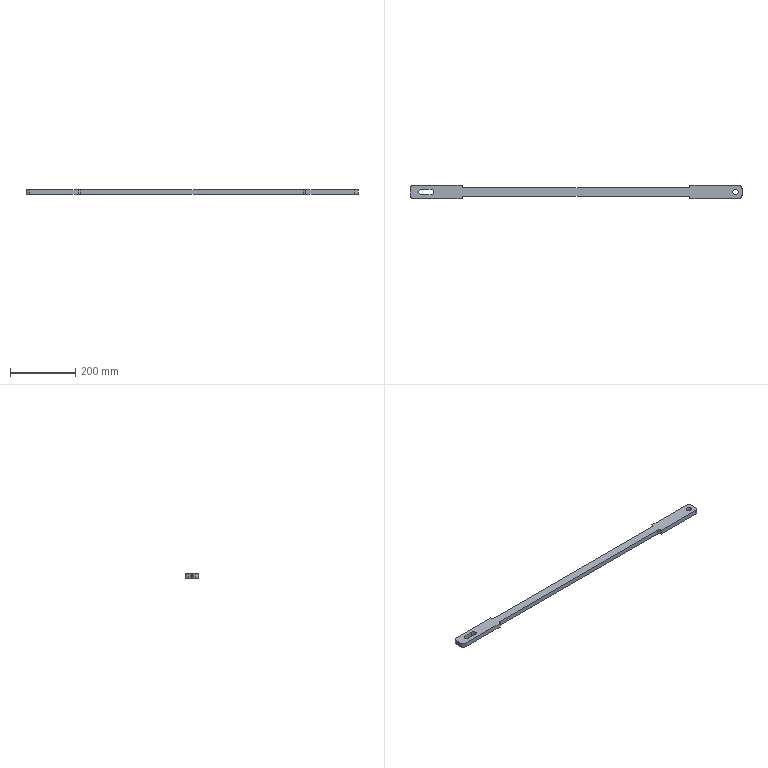Part | STEP file | Backup 2012-3-22-020 | 1 solid | 27 faces | box 1020 x 40 x 14 mm | volume 410338 mm3 | cylinder 15 | plane 12 | commonest cylinder face diameters 16 x5 15 x4 20 x4 6.8 x2